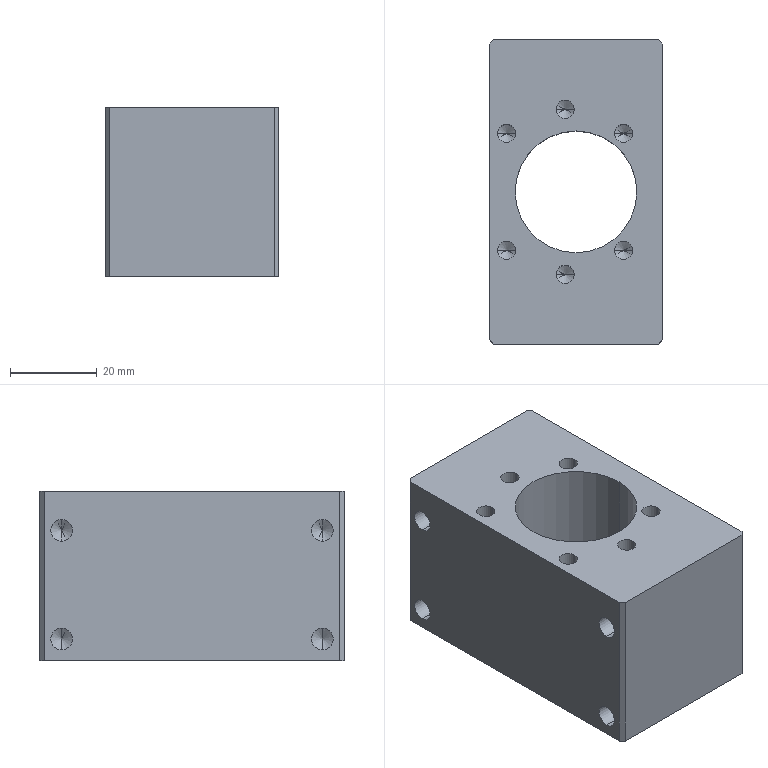Part | STEP file | 001-008-Traverse module nut seat | 1 solid | 52 faces | box 40 x 70 x 39 mm | volume 82202 mm3 | cylinder 22 | cone 20 | plane 10 | commonest cylinder face diameters 4.2 x12 5 x8 28 x2